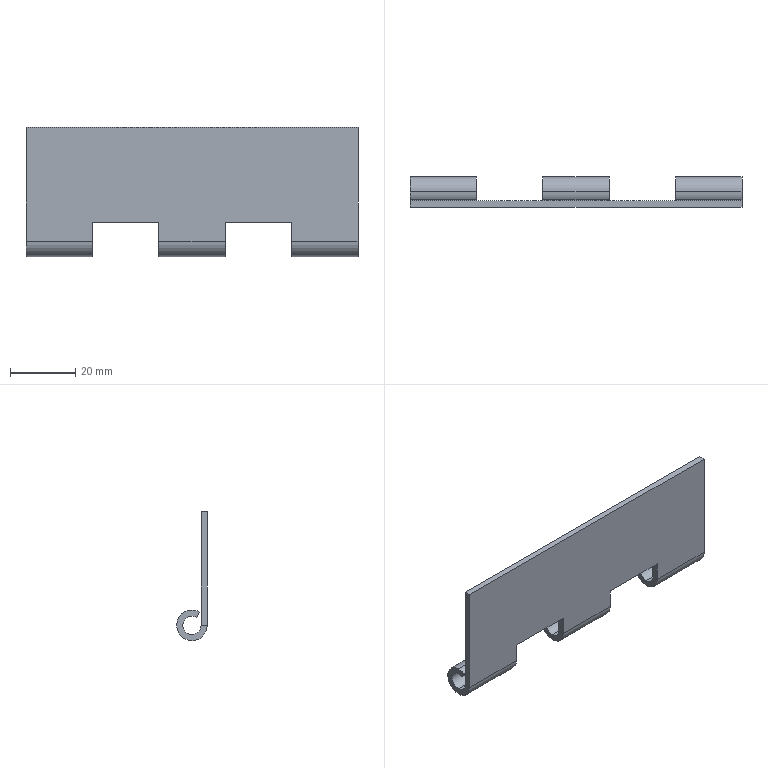Part | SolidWorks | features FlatPattern 1, ICE 1, SMBaseFlange 1, SheetMetal 1 | 1 solid | 36 faces | box 102 x 9.4 x 39.7 mm | volume 8617 mm3 | cylinder 18 | plane 18 | commonest cylinder face diameters 5.6 x9 9.4 x9
STEP:
#1=CARTESIAN_POINT('',(51.,1.9,-35.));
#2=VERTEX_POINT('',#1);
#3=CARTESIAN_POINT('',(51.,4.7,-37.8));
#4=VERTEX_POINT('',#3);
#5=CARTESIAN_POINT('',(51.,4.7,-35.));
#6=DIRECTION('',(1.,0.,0.));
#7=DIRECTION('',(0.,0.,-1.));
#8=AXIS2_PLACEMENT_3D('',#5,#6,#7);
#9=CIRCLE('',#8,2.8);
#10=EDGE_CURVE('',#2,#4,#9,.T.);
#11=ORIENTED_EDGE('',*,*,#10,.T.);
#12=CARTESIAN_POINT('',(30.6,4.7,-37.8));
#13=VERTEX_POINT('',#12);
#14=CARTESIAN_POINT('',(51.,4.7,-37.8));
#15=DIRECTION('',(-1.,0.,0.));
#16=VECTOR('',#15,1000.);
#17=LINE('',#14,#16);
#18=EDGE_CURVE('',#4,#13,#17,.T.);
#19=ORIENTED_EDGE('',*,*,#18,.T.);
#20=CARTESIAN_POINT('',(30.6,1.9,-35.));
#21=VERTEX_POINT('',#20);
#22=CARTESIAN_POINT('',(30.6,4.7,-35.));
#23=DIRECTION('',(1.,0.,0.));
#24=DIRECTION('',(0.,0.,-1.));
#25=AXIS2_PLACEMENT_3D('',#22,#23,#24);
#26=CIRCLE('',#25,2.8);
#27=EDGE_CURVE('',#21,#13,#26,.T.);
#28=ORIENTED_EDGE('',*,*,#27,.F.);
#29=CARTESIAN_POINT('',(51.,1.9,-35.));
#30=DIRECTION('',(-1.,0.,0.));
#31=VECTOR('',#30,1000.);
#32=LINE('',#29,#31);
#33=EDGE_CURVE('',#2,#21,#32,.T.);
#34=ORIENTED_EDGE('',*,*,#33,.F.);
#35=EDGE_LOOP('',(#11,#19,#28,#34));
#36=FACE_OUTER_BOUND('',#35,.T.);
#37=CARTESIAN_POINT('',(51.,4.7,-35.));
#38=DIRECTION('',(-1.,0.,0.));
#39=DIRECTION('',(0.,0.,1.));
#40=AXIS2_PLACEMENT_3D('',#37,#38,#39);
#41=CYLINDRICAL_SURFACE('',#40,2.8);
#42=ADVANCED_FACE('',(#36),#41,.F.);
#43=ORIENTED_EDGE('',*,*,#18,.F.);
#44=CARTESIAN_POINT('',(51.,4.7,-32.2));
#45=VERTEX_POINT('',#44);
#46=CARTESIAN_POINT('',(51.,4.7,-35.));
#47=DIRECTION('',(1.,0.,0.));
#48=DIRECTION('',(0.,0.,-1.));
#49=AXIS2_PLACEMENT_3D('',#46,#47,#48);
#50=CIRCLE('',#49,2.8);
#51=EDGE_CURVE('',#4,#45,#50,.T.);
#52=ORIENTED_EDGE('',*,*,#51,.T.);
#53=CARTESIAN_POINT('',(30.6,4.7,-32.2));
#54=VERTEX_POINT('',#53);
#55=CARTESIAN_POINT('',(51.,4.7,-32.2));
#56=DIRECTION('',(-1.,0.,0.));
#57=VECTOR('',#56,1000.);
#58=LINE('',#55,#57);
#59=EDGE_CURVE('',#45,#54,#58,.T.);
#60=ORIENTED_EDGE('',*,*,#59,.T.);
#61=CARTESIAN_POINT('',(30.6,4.7,-35.));
#62=DIRECTION('',(1.,0.,0.));
#63=DIRECTION('',(0.,0.,-1.));
#64=AXIS2_PLACEMENT_3D('',#61,#62,#63);
#65=CIRCLE('',#64,2.8);
#66=EDGE_CURVE('',#13,#54,#65,.T.);
#67=ORIENTED_EDGE('',*,*,#66,.F.);
#68=EDGE_LOOP('',(#43,#52,#60,#67));
#69=FACE_OUTER_BOUND('',#68,.T.);
#70=CARTESIAN_POINT('',(51.,4.7,-35.));
#71=DIRECTION('',(-1.,0.,0.));
#72=DIRECTION('',(0.,0.,1.));
#73=AXIS2_PLACEMENT_3D('',#70,#71,#72);
#74=CYLINDRICAL_SURFACE('',#73,2.8);
#75=ADVANCED_FACE('',(#69),#74,.F.);
#76=CARTESIAN_POINT('',(51.,4.7,-39.7));
#77=VERTEX_POINT('',#76);
#78=CARTESIAN_POINT('',(51.,4.7,-30.3));
#79=VERTEX_POINT('',#78);
#80=CARTESIAN_POINT('',(51.,4.7,-35.));
#81=DIRECTION('',(1.,0.,0.));
#82=DIRECTION('',(0.,0.,-1.));
#83=AXIS2_PLACEMENT_3D('',#80,#81,#82);
#84=CIRCLE('',#83,4.7);
#85=EDGE_CURVE('',#77,#79,#84,.T.);
#86=ORIENTED_EDGE('',*,*,#85,.F.);
#87=CARTESIAN_POINT('',(30.6,4.7,-39.7));
#88=VERTEX_POINT('',#87);
#89=CARTESIAN_POINT('',(51.,4.7,-39.7));
#90=DIRECTION('',(-1.,0.,0.));
#91=VECTOR('',#90,1000.);
#92=LINE('',#89,#91);
#93=EDGE_CURVE('',#77,#88,#92,.T.);
#94=ORIENTED_EDGE('',*,*,#93,.T.);
#95=CARTESIAN_POINT('',(30.6,4.7,-30.3));
#96=VERTEX_POINT('',#95);
#97=CARTESIAN_POINT('',(30.6,4.7,-35.));
#98=DIRECTION('',(1.,0.,0.));
#99=DIRECTION('',(0.,0.,-1.));
#100=AXIS2_PLACEMENT_3D('',#97,#98,#99);
#101=CIRCLE('',#100,4.7);
#102=EDGE_CURVE('',#88,#96,#101,.T.);
#103=ORIENTED_EDGE('',*,*,#102,.T.);
#104=CARTESIAN_POINT('',(51.,4.7,-30.3));
#105=DIRECTION('',(-1.,0.,0.));
#106=VECTOR('',#105,1000.);
#107=LINE('',#104,#106);
#108=EDGE_CURVE('',#79,#96,#107,.T.);
#109=ORIENTED_EDGE('',*,*,#108,.F.);
#110=EDGE_LOOP('',(#86,#94,#103,#109));
#111=FACE_OUTER_BOUND('',#110,.T.);
#112=CARTESIAN_POINT('',(51.,4.7,-35.));
#113=DIRECTION('',(-1.,0.,0.));
#114=DIRECTION('',(0.,0.,1.));
#115=AXIS2_PLACEMENT_3D('',#112,#113,#114);
#116=CYLINDRICAL_SURFACE('',#115,4.7);
#117=ADVANCED_FACE('',(#111),#116,.T.);
#118=CARTESIAN_POINT('',(51.,2.35,-30.93));
#119=VERTEX_POINT('',#118);
#120=CARTESIAN_POINT('',(51.,4.7,-35.));
#121=DIRECTION('',(1.,0.,0.));
#122=DIRECTION('',(0.,0.,-1.));
#123=AXIS2_PLACEMENT_3D('',#120,#121,#122);
#124=CIRCLE('',#123,4.7);
#125=EDGE_CURVE('',#79,#119,#124,.T.);
#126=ORIENTED_EDGE('',*,*,#125,.F.);
#127=ORIENTED_EDGE('',*,*,#108,.T.);
#128=CARTESIAN_POINT('',(30.6,2.35,-30.93));
#129=VERTEX_POINT('',#128);
#130=CARTESIAN_POINT('',(30.6,4.7,-35.));
#131=DIRECTION('',(1.,0.,0.));
#132=DIRECTION('',(0.,0.,-1.));
#133=AXIS2_PLACEMENT_3D('',#130,#131,#132);
#134=CIRCLE('',#133,4.7);
#135=EDGE_CURVE('',#96,#129,#134,.T.);
#136=ORIENTED_EDGE('',*,*,#135,.T.);
#137=CARTESIAN_POINT('',(51.,2.35,-30.93));
#138=DIRECTION('',(-1.,0.,0.));
#139=VECTOR('',#138,1000.);
#140=LINE('',#137,#139);
#141=EDGE_CURVE('',#119,#129,#140,.T.);
#142=ORIENTED_EDGE('',*,*,#141,.F.);
#143=EDGE_LOOP('',(#126,#127,#136,#142));
#144=FACE_OUTER_BOUND('',#143,.T.);
#145=CARTESIAN_POINT('',(51.,4.7,-35.));
#146=DIRECTION('',(-1.,0.,0.));
#147=DIRECTION('',(0.,0.,1.));
#148=AXIS2_PLACEMENT_3D('',#145,#146,#147);
#149=CYLINDRICAL_SURFACE('',#148,4.7);
#150=ADVANCED_FACE('',(#144),#149,.T.);
#151=CARTESIAN_POINT('',(10.2,4.7,-37.8));
#152=VERTEX_POINT('',#151);
#153=CARTESIAN_POINT('',(10.2,1.9,-35.));
#154=VERTEX_POINT('',#153);
#155=CARTESIAN_POINT('',(10.2,4.7,-35.));
#156=DIRECTION('',(-1.,0.,0.));
#157=DIRECTION('',(0.,0.,1.));
#158=AXIS2_PLACEMENT_3D('',#155,#156,#157);
#159=CIRCLE('',#158,2.8);
#160=EDGE_CURVE('',#152,#154,#159,.T.);
#161=ORIENTED_EDGE('',*,*,#160,.F.);
#162=CARTESIAN_POINT('',(-10.2,4.7,-37.8));
#163=VERTEX_POINT('',#162);
#164=CARTESIAN_POINT('',(51.,4.7,-37.8));
#165=DIRECTION('',(-1.,0.,0.));
#166=VECTOR('',#165,1000.);
#167=LINE('',#164,#166);
#168=EDGE_CURVE('',#152,#163,#167,.T.);
#169=ORIENTED_EDGE('',*,*,#168,.T.);
#170=CARTESIAN_POINT('',(-10.2,1.9,-35.));
#171=VERTEX_POINT('',#170);
#172=CARTESIAN_POINT('',(-10.2,4.7,-35.));
#173=DIRECTION('',(1.,0.,0.));
#174=DIRECTION('',(0.,0.,-1.));
#175=AXIS2_PLACEMENT_3D('',#172,#173,#174);
#176=CIRCLE('',#175,2.8);
#177=EDGE_CURVE('',#171,#163,#176,.T.);
#178=ORIENTED_EDGE('',*,*,#177,.F.);
#179=CARTESIAN_POINT('',(51.,1.9,-35.));
#180=DIRECTION('',(-1.,0.,0.));
#181=VECTOR('',#180,1000.);
#182=LINE('',#179,#181);
#183=EDGE_CURVE('',#154,#171,#182,.T.);
#184=ORIENTED_EDGE('',*,*,#183,.F.);
#185=EDGE_LOOP('',(#161,#169,#178,#184));
#186=FACE_OUTER_BOUND('',#185,.T.);
#187=CARTESIAN_POINT('',(51.,4.7,-35.));
#188=DIRECTION('',(-1.,0.,0.));
#189=DIRECTION('',(0.,0.,1.));
#190=AXIS2_PLACEMENT_3D('',#187,#188,#189);
#191=CYLINDRICAL_SURFACE('',#190,2.8);
#192=ADVANCED_FACE('',(#186),#191,.F.);
#193=ORIENTED_EDGE('',*,*,#168,.F.);
#194=CARTESIAN_POINT('',(10.2,4.7,-32.2));
#195=VERTEX_POINT('',#194);
#196=CARTESIAN_POINT('',(10.2,4.7,-35.));
#197=DIRECTION('',(-1.,0.,0.));
#198=DIRECTION('',(0.,0.,1.));
#199=AXIS2_PLACEMENT_3D('',#196,#197,#198);
#200=CIRCLE('',#199,2.8);
#201=EDGE_CURVE('',#195,#152,#200,.T.);
#202=ORIENTED_EDGE('',*,*,#201,.F.);
#203=CARTESIAN_POINT('',(-10.2,4.7,-32.2));
#204=VERTEX_POINT('',#203);
#205=CARTESIAN_POINT('',(51.,4.7,-32.2));
#206=DIRECTION('',(-1.,0.,0.));
#207=VECTOR('',#206,1000.);
#208=LINE('',#205,#207);
#209=EDGE_CURVE('',#195,#204,#208,.T.);
#210=ORIENTED_EDGE('',*,*,#209,.T.);
#211=CARTESIAN_POINT('',(-10.2,4.7,-35.));
#212=DIRECTION('',(1.,0.,0.));
#213=DIRECTION('',(0.,0.,-1.));
#214=AXIS2_PLACEMENT_3D('',#211,#212,#213);
#215=CIRCLE('',#214,2.8);
#216=EDGE_CURVE('',#163,#204,#215,.T.);
#217=ORIENTED_EDGE('',*,*,#216,.F.);
#218=EDGE_LOOP('',(#193,#202,#210,#217));
#219=FACE_OUTER_BOUND('',#218,.T.);
#220=CARTESIAN_POINT('',(51.,4.7,-35.));
#221=DIRECTION('',(-1.,0.,0.));
#222=DIRECTION('',(0.,0.,1.));
#223=AXIS2_PLACEMENT_3D('',#220,#221,#222);
#224=CYLINDRICAL_SURFACE('',#223,2.8);
#225=ADVANCED_FACE('',(#219),#224,.F.);
#226=CARTESIAN_POINT('',(-30.6,4.7,-37.8));
#227=VERTEX_POINT('',#226);
#228=CARTESIAN_POINT('',(-30.6,1.9,-35.));
#229=VERTEX_POINT('',#228);
#230=CARTESIAN_POINT('',(-30.6,4.7,-35.));
#231=DIRECTION('',(-1.,0.,0.));
#232=DIRECTION('',(0.,0.,1.));
#233=AXIS2_PLACEMENT_3D('',#230,#231,#232);
#234=CIRCLE('',#233,2.8);
#235=EDGE_CURVE('',#227,#229,#234,.T.);
#236=ORIENTED_EDGE('',*,*,#235,.F.);
#237=CARTESIAN_POINT('',(-51.,4.7,-37.8));
#238=VERTEX_POINT('',#237);
#239=CARTESIAN_POINT('',(51.,4.7,-37.8));
#240=DIRECTION('',(-1.,0.,0.));
#241=VECTOR('',#240,1000.);
#242=LINE('',#239,#241);
#243=EDGE_CURVE('',#227,#238,#242,.T.);
#244=ORIENTED_EDGE('',*,*,#243,.T.);
#245=CARTESIAN_POINT('',(-51.,1.9,-35.));
#246=VERTEX_POINT('',#245);
#247=CARTESIAN_POINT('',(-51.,4.7,-35.));
#248=DIRECTION('',(1.,0.,0.));
#249=DIRECTION('',(0.,0.,-1.));
#250=AXIS2_PLACEMENT_3D('',#247,#248,#249);
#251=CIRCLE('',#250,2.8);
#252=EDGE_CURVE('',#246,#238,#251,.T.);
#253=ORIENTED_EDGE('',*,*,#252,.F.);
#254=CARTESIAN_POINT('',(51.,1.9,-35.));
#255=DIRECTION('',(-1.,0.,0.));
#256=VECTOR('',#255,1000.);
#257=LINE('',#254,#256);
#258=EDGE_CURVE('',#229,#246,#257,.T.);
#259=ORIENTED_EDGE('',*,*,#258,.F.);
#260=EDGE_LOOP('',(#236,#244,#253,#259));
#261=FACE_OUTER_BOUND('',#260,.T.);
#262=CARTESIAN_POINT('',(51.,4.7,-35.));
#263=DIRECTION('',(-1.,0.,0.));
#264=DIRECTION('',(0.,0.,1.));
#265=AXIS2_PLACEMENT_3D('',#262,#263,#264);
#266=CYLINDRICAL_SURFACE('',#265,2.8);
#267=ADVANCED_FACE('',(#261),#266,.F.);
#268=ORIENTED_EDGE('',*,*,#243,.F.);
#269=CARTESIAN_POINT('',(-30.6,4.7,-32.2));
#270=VERTEX_POINT('',#269);
#271=CARTESIAN_POINT('',(-30.6,4.7,-35.));
#272=DIRECTION('',(-1.,0.,0.));
#273=DIRECTION('',(0.,0.,1.));
#274=AXIS2_PLACEMENT_3D('',#271,#272,#273);
#275=CIRCLE('',#274,2.8);
#276=EDGE_CURVE('',#270,#227,#275,.T.);
#277=ORIENTED_EDGE('',*,*,#276,.F.);
#278=CARTESIAN_POINT('',(-51.,4.7,-32.2));
#279=VERTEX_POINT('',#278);
#280=CARTESIAN_POINT('',(51.,4.7,-32.2));
#281=DIRECTION('',(-1.,0.,0.));
#282=VECTOR('',#281,1000.);
#283=LINE('',#280,#282);
#284=EDGE_CURVE('',#270,#279,#283,.T.);
#285=ORIENTED_EDGE('',*,*,#284,.T.);
#286=CARTESIAN_POINT('',(-51.,4.7,-35.));
#287=DIRECTION('',(1.,0.,0.));
#288=DIRECTION('',(0.,0.,-1.));
#289=AXIS2_PLACEMENT_3D('',#286,#287,#288);
#290=CIRCLE('',#289,2.8);
#291=EDGE_CURVE('',#238,#279,#290,.T.);
#292=ORIENTED_EDGE('',*,*,#291,.F.);
#293=EDGE_LOOP('',(#268,#277,#285,#292));
#294=FACE_OUTER_BOUND('',#293,.T.);
#295=CARTESIAN_POINT('',(51.,4.7,-35.));
#296=DIRECTION('',(-1.,0.,0.));
#297=DIRECTION('',(0.,0.,1.));
#298=AXIS2_PLACEMENT_3D('',#295,#296,#297);
#299=CYLINDRICAL_SURFACE('',#298,2.8);
#300=ADVANCED_FACE('',(#294),#299,.F.);
#301=CARTESIAN_POINT('',(10.2,4.7,-30.3));
#302=VERTEX_POINT('',#301);
#303=CARTESIAN_POINT('',(10.2,4.7,-39.7));
#304=VERTEX_POINT('',#303);
#305=CARTESIAN_POINT('',(10.2,4.7,-35.));
#306=DIRECTION('',(-1.,0.,0.));
#307=DIRECTION('',(0.,0.,1.));
#308=AXIS2_PLACEMENT_3D('',#305,#306,#307);
#309=CIRCLE('',#308,4.7);
#310=EDGE_CURVE('',#302,#304,#309,.T.);
#311=ORIENTED_EDGE('',*,*,#310,.T.);
#312=CARTESIAN_POINT('',(-10.2,4.7,-39.7));
#313=VERTEX_POINT('',#312);
#314=CARTESIAN_POINT('',(51.,4.7,-39.7));
#315=DIRECTION('',(-1.,0.,0.));
#316=VECTOR('',#315,1000.);
#317=LINE('',#314,#316);
#318=EDGE_CURVE('',#304,#313,#317,.T.);
#319=ORIENTED_EDGE('',*,*,#318,.T.);
#320=CARTESIAN_POINT('',(-10.2,4.7,-30.3));
#321=VERTEX_POINT('',#320);
#322=CARTESIAN_POINT('',(-10.2,4.7,-35.));
#323=DIRECTION('',(1.,0.,0.));
#324=DIRECTION('',(0.,0.,-1.));
#325=AXIS2_PLACEMENT_3D('',#322,#323,#324);
#326=CIRCLE('',#325,4.7);
#327=EDGE_CURVE('',#313,#321,#326,.T.);
#328=ORIENTED_EDGE('',*,*,#327,.T.);
#329=CARTESIAN_POINT('',(51.,4.7,-30.3));
#330=DIRECTION('',(-1.,0.,0.));
#331=VECTOR('',#330,1000.);
#332=LINE('',#329,#331);
#333=EDGE_CURVE('',#302,#321,#332,.T.);
#334=ORIENTED_EDGE('',*,*,#333,.F.);
#335=EDGE_LOOP('',(#311,#319,#328,#334));
#336=FACE_OUTER_BOUND('',#335,.T.);
#337=CARTESIAN_POINT('',(51.,4.7,-35.));
#338=DIRECTION('',(-1.,0.,0.));
#339=DIRECTION('',(0.,0.,1.));
#340=AXIS2_PLACEMENT_3D('',#337,#338,#339);
#341=CYLINDRICAL_SURFACE('',#340,4.7);
#342=ADVANCED_FACE('',(#336),#341,.T.);
#343=CARTESIAN_POINT('',(10.2,2.35,-30.93));
#344=VERTEX_POINT('',#343);
#345=CARTESIAN_POINT('',(10.2,4.7,-35.));
#346=DIRECTION('',(-1.,0.,0.));
#347=DIRECTION('',(0.,0.,1.));
#348=AXIS2_PLACEMENT_3D('',#345,#346,#347);
#349=CIRCLE('',#348,4.7);
#350=EDGE_CURVE('',#344,#302,#349,.T.);
#351=ORIENTED_EDGE('',*,*,#350,.T.);
#352=ORIENTED_EDGE('',*,*,#333,.T.);
#353=CARTESIAN_POINT('',(-10.2,2.35,-30.93));
#354=VERTEX_POINT('',#353);
#355=CARTESIAN_POINT('',(-10.2,4.7,-35.));
#356=DIRECTION('',(1.,0.,0.));
#357=DIRECTION('',(0.,0.,-1.));
#358=AXIS2_PLACEMENT_3D('',#355,#356,#357);
#359=CIRCLE('',#358,4.7);
#360=EDGE_CURVE('',#321,#354,#359,.T.);
#361=ORIENTED_EDGE('',*,*,#360,.T.);
#362=CARTESIAN_POINT('',(51.,2.35,-30.93));
#363=DIRECTION('',(-1.,0.,0.));
#364=VECTOR('',#363,1000.);
#365=LINE('',#362,#364);
#366=EDGE_CURVE('',#344,#354,#365,.T.);
#367=ORIENTED_EDGE('',*,*,#366,.F.);
#368=EDGE_LOOP('',(#351,#352,#361,#367));
#369=FACE_OUTER_BOUND('',#368,.T.);
#370=CARTESIAN_POINT('',(51.,4.7,-35.));
#371=DIRECTION('',(-1.,0.,0.));
#372=DIRECTION('',(0.,0.,1.));
#373=AXIS2_PLACEMENT_3D('',#370,#371,#372);
#374=CYLINDRICAL_SURFACE('',#373,4.7);
#375=ADVANCED_FACE('',(#369),#374,.T.);
#376=CARTESIAN_POINT('',(-30.6,4.7,-30.3));
#377=VERTEX_POINT('',#376);
#378=CARTESIAN_POINT('',(-30.6,4.7,-39.7));
#379=VERTEX_POINT('',#378);
#380=CARTESIAN_POINT('',(-30.6,4.7,-35.));
#381=DIRECTION('',(-1.,0.,0.));
#382=DIRECTION('',(0.,0.,1.));
#383=AXIS2_PLACEMENT_3D('',#380,#381,#382);
#384=CIRCLE('',#383,4.7);
#385=EDGE_CURVE('',#377,#379,#384,.T.);
#386=ORIENTED_EDGE('',*,*,#385,.T.);
#387=CARTESIAN_POINT('',(-51.,4.7,-39.7));
#388=VERTEX_POINT('',#387);
#389=CARTESIAN_POINT('',(51.,4.7,-39.7));
#390=DIRECTION('',(-1.,0.,0.));
#391=VECTOR('',#390,1000.);
#392=LINE('',#389,#391);
#393=EDGE_CURVE('',#379,#388,#392,.T.);
#394=ORIENTED_EDGE('',*,*,#393,.T.);
#395=CARTESIAN_POINT('',(-51.,4.7,-30.3));
#396=VERTEX_POINT('',#395);
#397=CARTESIAN_POINT('',(-51.,4.7,-35.));
#398=DIRECTION('',(1.,0.,0.));
#399=DIRECTION('',(0.,0.,-1.));
#400=AXIS2_PLACEMENT_3D('',#397,#398,#399);
#401=CIRCLE('',#400,4.7);
#402=EDGE_CURVE('',#388,#396,#401,.T.);
#403=ORIENTED_EDGE('',*,*,#402,.T.);
#404=CARTESIAN_POINT('',(51.,4.7,-30.3));
#405=DIRECTION('',(-1.,0.,0.));
#406=VECTOR('',#405,1000.);
#407=LINE('',#404,#406);
#408=EDGE_CURVE('',#377,#396,#407,.T.);
#409=ORIENTED_EDGE('',*,*,#408,.F.);
#410=EDGE_LOOP('',(#386,#394,#403,#409));
#411=FACE_OUTER_BOUND('',#410,.T.);
#412=CARTESIAN_POINT('',(51.,4.7,-35.));
#413=DIRECTION('',(-1.,0.,0.));
#414=DIRECTION('',(0.,0.,1.));
#415=AXIS2_PLACEMENT_3D('',#412,#413,#414);
#416=CYLINDRICAL_SURFACE('',#415,4.7);
#417=ADVANCED_FACE('',(#411),#416,.T.);
#418=CARTESIAN_POINT('',(-30.6,2.35,-30.93));
#419=VERTEX_POINT('',#418);
#420=CARTESIAN_POINT('',(-30.6,4.7,-35.));
#421=DIRECTION('',(-1.,0.,0.));
#422=DIRECTION('',(0.,0.,1.));
#423=AXIS2_PLACEMENT_3D('',#420,#421,#422);
#424=CIRCLE('',#423,4.7);
#425=EDGE_CURVE('',#419,#377,#424,.T.);
#426=ORIENTED_EDGE('',*,*,#425,.T.);
#427=ORIENTED_EDGE('',*,*,#408,.T.);
#428=CARTESIAN_POINT('',(-51.,2.35,-30.93));
#429=VERTEX_POINT('',#428);
#430=CARTESIAN_POINT('',(-51.,4.7,-35.));
#431=DIRECTION('',(1.,0.,0.));
#432=DIRECTION('',(0.,0.,-1.));
#433=AXIS2_PLACEMENT_3D('',#430,#431,#432);
#434=CIRCLE('',#433,4.7);
#435=EDGE_CURVE('',#396,#429,#434,.T.);
#436=ORIENTED_EDGE('',*,*,#435,.T.);
#437=CARTESIAN_POINT('',(51.,2.35,-30.93));
#438=DIRECTION('',(-1.,0.,0.));
#439=VECTOR('',#438,1000.);
#440=LINE('',#437,#439);
#441=EDGE_CURVE('',#419,#429,#440,.T.);
#442=ORIENTED_EDGE('',*,*,#441,.F.);
#443=EDGE_LOOP('',(#426,#427,#436,#442));
#444=FACE_OUTER_BOUND('',#443,.T.);
#445=CARTESIAN_POINT('',(51.,4.7,-35.));
#446=DIRECTION('',(-1.,0.,0.));
#447=DIRECTION('',(0.,0.,1.));
#448=AXIS2_PLACEMENT_3D('',#445,#446,#447);
#449=CYLINDRICAL_SURFACE('',#448,4.7);
#450=ADVANCED_FACE('',(#444),#449,.T.);
#451=CARTESIAN_POINT('',(-10.2,1.9,-29.2));
#452=VERTEX_POINT('',#451);
#453=CARTESIAN_POINT('',(-10.2,1.9,0.));
#454=DIRECTION('',(0.,0.,-1.));
#455=VECTOR('',#454,1000.);
#456=LINE('',#453,#455);
#457=EDGE_CURVE('',#452,#171,#456,.T.);
#458=ORIENTED_EDGE('',*,*,#457,.T.);
#459=CARTESIAN_POINT('',(-10.2,0.,-35.));
#460=VERTEX_POINT('',#459);
#461=CARTESIAN_POINT('',(-10.2,1.9,-35.));
#462=DIRECTION('',(0.,-1.,0.));
#463=VECTOR('',#462,1000.);
#464=LINE('',#461,#463);
#465=EDGE_CURVE('',#171,#460,#464,.T.);
#466=ORIENTED_EDGE('',*,*,#465,.T.);
#467=CARTESIAN_POINT('',(-10.2,0.,-29.2));
#468=VERTEX_POINT('',#467);
#469=CARTESIAN_POINT('',(-10.2,0.,0.));
#470=DIRECTION('',(0.,0.,-1.));
#471=VECTOR('',#470,1000.);
#472=LINE('',#469,#471);
#473=EDGE_CURVE('',#468,#460,#472,.T.);
#474=ORIENTED_EDGE('',*,*,#473,.F.);
#475=CARTESIAN_POINT('',(-10.2,9.4,-29.2));
#476=DIRECTION('',(0.,-1.,0.));
#477=VECTOR('',#476,1000.);
#478=LINE('',#475,#477);
#479=EDGE_CURVE('',#452,#468,#478,.T.);
#480=ORIENTED_EDGE('',*,*,#479,.F.);
#481=EDGE_LOOP('',(#458,#466,#474,#480));
#482=FACE_OUTER_BOUND('',#481,.T.);
#483=CARTESIAN_POINT('',(-10.2,9.4,-39.7));
#484=DIRECTION('',(1.,0.,0.));
#485=DIRECTION('',(0.,0.,-1.));
#486=AXIS2_PLACEMENT_3D('',#483,#484,#485);
#487=PLANE('',#486);
#488=ADVANCED_FACE('',(#482),#487,.F.);
#489=CARTESIAN_POINT('',(30.6,1.9,-29.2));
#490=VERTEX_POINT('',#489);
#491=CARTESIAN_POINT('',(30.6,1.9,0.));
#492=DIRECTION('',(0.,0.,-1.));
#493=VECTOR('',#492,1000.);
#494=LINE('',#491,#493);
#495=EDGE_CURVE('',#490,#21,#494,.T.);
#496=ORIENTED_EDGE('',*,*,#495,.T.);
#497=CARTESIAN_POINT('',(30.6,0.,-35.));
#498=VERTEX_POINT('',#497);
#499=CARTESIAN_POINT('',(30.6,1.9,-35.));
#500=DIRECTION('',(0.,-1.,0.));
#501=VECTOR('',#500,1000.);
#502=LINE('',#499,#501);
#503=EDGE_CURVE('',#21,#498,#502,.T.);
#504=ORIENTED_EDGE('',*,*,#503,.T.);
#505=CARTESIAN_POINT('',(30.6,0.,-29.2));
#506=VERTEX_POINT('',#505);
#507=CARTESIAN_POINT('',(30.6,0.,0.));
#508=DIRECTION('',(0.,0.,-1.));
#509=VECTOR('',#508,1000.);
#510=LINE('',#507,#509);
#511=EDGE_CURVE('',#506,#498,#510,.T.);
#512=ORIENTED_EDGE('',*,*,#511,.F.);
#513=CARTESIAN_POINT('',(30.6,9.4,-29.2));
#514=DIRECTION('',(0.,-1.,0.));
#515=VECTOR('',#514,1000.);
#516=LINE('',#513,#515);
#517=EDGE_CURVE('',#490,#506,#516,.T.);
#518=ORIENTED_EDGE('',*,*,#517,.F.);
#519=EDGE_LOOP('',(#496,#504,#512,#518));
#520=FACE_OUTER_BOUND('',#519,.T.);
#521=CARTESIAN_POINT('',(30.6,9.4,-39.7));
#522=DIRECTION('',(1.,0.,0.));
#523=DIRECTION('',(0.,0.,-1.));
#524=AXIS2_PLACEMENT_3D('',#521,#522,#523);
#525=PLANE('',#524);
#526=ADVANCED_FACE('',(#520),#525,.F.);
#527=ORIENTED_EDGE('',*,*,#393,.F.);
#528=CARTESIAN_POINT('',(-30.6,0.,-35.));
#529=VERTEX_POINT('',#528);
#530=CARTESIAN_POINT('',(-30.6,4.7,-35.));
#531=DIRECTION('',(-1.,0.,0.));
#532=DIRECTION('',(0.,0.,1.));
#533=AXIS2_PLACEMENT_3D('',#530,#531,#532);
#534=CIRCLE('',#533,4.7);
#535=EDGE_CURVE('',#379,#529,#534,.T.);
#536=ORIENTED_EDGE('',*,*,#535,.T.);
#537=CARTESIAN_POINT('',(-51.,0.,-35.));
#538=VERTEX_POINT('',#537);
#539=CARTESIAN_POINT('',(51.,0.,-35.));
#540=DIRECTION('',(-1.,0.,0.));
#541=VECTOR('',#540,1000.);
#542=LINE('',#539,#541);
#543=EDGE_CURVE('',#529,#538,#542,.T.);
#544=ORIENTED_EDGE('',*,*,#543,.T.);
#545=CARTESIAN_POINT('',(-51.,4.7,-35.));
#546=DIRECTION('',(1.,0.,0.));
#547=DIRECTION('',(0.,0.,-1.));
#548=AXIS2_PLACEMENT_3D('',#545,#546,#547);
#549=CIRCLE('',#548,4.7);
#550=EDGE_CURVE('',#538,#388,#549,.T.);
#551=ORIENTED_EDGE('',*,*,#550,.T.);
#552=EDGE_LOOP('',(#527,#536,#544,#551));
#553=FACE_OUTER_BOUND('',#552,.T.);
#554=CARTESIAN_POINT('',(51.,4.7,-35.));
#555=DIRECTION('',(-1.,0.,0.));
#556=DIRECTION('',(0.,0.,1.));
#557=AXIS2_PLACEMENT_3D('',#554,#555,#556);
#558=CYLINDRICAL_SURFACE('',#557,4.7);
#559=ADVANCED_FACE('',(#553),#558,.T.);
#560=ORIENTED_EDGE('',*,*,#318,.F.);
#561=CARTESIAN_POINT('',(10.2,0.,-35.));
#562=VERTEX_POINT('',#561);
#563=CARTESIAN_POINT('',(10.2,4.7,-35.));
#564=DIRECTION('',(-1.,0.,0.));
#565=DIRECTION('',(0.,0.,1.));
#566=AXIS2_PLACEMENT_3D('',#563,#564,#565);
#567=CIRCLE('',#566,4.7);
#568=EDGE_CURVE('',#304,#562,#567,.T.);
#569=ORIENTED_EDGE('',*,*,#568,.T.);
#570=CARTESIAN_POINT('',(51.,0.,-35.));
#571=DIRECTION('',(-1.,0.,0.));
#572=VECTOR('',#571,1000.);
#573=LINE('',#570,#572);
#574=EDGE_CURVE('',#562,#460,#573,.T.);
#575=ORIENTED_EDGE('',*,*,#574,.T.);
#576=CARTESIAN_POINT('',(-10.2,4.7,-35.));
#577=DIRECTION('',(1.,0.,0.));
#578=DIRECTION('',(0.,0.,-1.));
#579=AXIS2_PLACEMENT_3D('',#576,#577,#578);
#580=CIRCLE('',#579,4.7);
#581=EDGE_CURVE('',#460,#313,#580,.T.);
#582=ORIENTED_EDGE('',*,*,#581,.T.);
#583=EDGE_LOOP('',(#560,#569,#575,#582));
#584=FACE_OUTER_BOUND('',#583,.T.);
#585=CARTESIAN_POINT('',(51.,4.7,-35.));
#586=DIRECTION('',(-1.,0.,0.));
#587=DIRECTION('',(0.,0.,1.));
#588=AXIS2_PLACEMENT_3D('',#585,#586,#587);
#589=CYLINDRICAL_SURFACE('',#588,4.7);
#590=ADVANCED_FACE('',(#584),#589,.T.);
#591=CARTESIAN_POINT('',(-30.6,3.3,-32.575));
#592=VERTEX_POINT('',#591);
#593=CARTESIAN_POINT('',(-30.6,3.3,-32.575));
#594=DIRECTION('',(0.,0.5,-0.866));
#595=VECTOR('',#594,1000.);
#596=LINE('',#593,#595);
#597=EDGE_CURVE('',#419,#592,#596,.T.);
#598=ORIENTED_EDGE('',*,*,#597,.F.);
#599=ORIENTED_EDGE('',*,*,#441,.T.);
#600=CARTESIAN_POINT('',(-51.,3.3,-32.575));
#601=VERTEX_POINT('',#600);
#602=CARTESIAN_POINT('',(-51.,3.3,-32.575));
#603=DIRECTION('',(0.,-0.5,0.866));
#604=VECTOR('',#603,1000.);
#605=LINE('',#602,#604);
#606=EDGE_CURVE('',#601,#429,#605,.T.);
#607=ORIENTED_EDGE('',*,*,#606,.F.);
#608=CARTESIAN_POINT('',(51.,3.3,-32.575));
#609=DIRECTION('',(-1.,0.,0.));
#610=VECTOR('',#609,1000.);
#611=LINE('',#608,#610);
#612=EDGE_CURVE('',#592,#601,#611,.T.);
#613=ORIENTED_EDGE('',*,*,#612,.F.);
#614=EDGE_LOOP('',(#598,#599,#607,#613));
#615=FACE_OUTER_BOUND('',#614,.T.);
#616=CARTESIAN_POINT('',(51.,3.3,-32.575));
#617=DIRECTION('',(0.,-0.866,-0.5));
#618=DIRECTION('',(0.,0.5,-0.866));
#619=AXIS2_PLACEMENT_3D('',#616,#617,#618);
#620=PLANE('',#619);
#621=ADVANCED_FACE('',(#615),#620,.T.);
#622=CARTESIAN_POINT('',(-10.2,3.3,-32.575));
#623=VERTEX_POINT('',#622);
#624=CARTESIAN_POINT('',(-10.2,3.3,-32.575));
#625=DIRECTION('',(0.,-0.5,0.866));
#626=VECTOR('',#625,1000.);
#627=LINE('',#624,#626);
#628=EDGE_CURVE('',#623,#354,#627,.T.);
#629=ORIENTED_EDGE('',*,*,#628,.F.);
#630=CARTESIAN_POINT('',(10.2,3.3,-32.575));
#631=VERTEX_POINT('',#630);
#632=CARTESIAN_POINT('',(51.,3.3,-32.575));
#633=DIRECTION('',(-1.,0.,0.));
#634=VECTOR('',#633,1000.);
#635=LINE('',#632,#634);
#636=EDGE_CURVE('',#631,#623,#635,.T.);
#637=ORIENTED_EDGE('',*,*,#636,.F.);
#638=CARTESIAN_POINT('',(10.2,3.3,-32.575));
#639=DIRECTION('',(0.,0.5,-0.866));
#640=VECTOR('',#639,1000.);
#641=LINE('',#638,#640);
#642=EDGE_CURVE('',#344,#631,#641,.T.);
#643=ORIENTED_EDGE('',*,*,#642,.F.);
#644=ORIENTED_EDGE('',*,*,#366,.T.);
#645=EDGE_LOOP('',(#629,#637,#643,#644));
#646=FACE_OUTER_BOUND('',#645,.T.);
#647=CARTESIAN_POINT('',(51.,3.3,-32.575));
#648=DIRECTION('',(0.,-0.866,-0.5));
#649=DIRECTION('',(0.,0.5,-0.866));
#650=AXIS2_PLACEMENT_3D('',#647,#648,#649);
#651=PLANE('',#650);
#652=ADVANCED_FACE('',(#646),#651,.T.);
#653=ORIENTED_EDGE('',*,*,#284,.F.);
#654=CARTESIAN_POINT('',(-30.6,4.7,-35.));
#655=DIRECTION('',(-1.,0.,0.));
#656=DIRECTION('',(0.,0.,1.));
#657=AXIS2_PLACEMENT_3D('',#654,#655,#656);
#658=CIRCLE('',#657,2.8);
#659=EDGE_CURVE('',#592,#270,#658,.T.);
#660=ORIENTED_EDGE('',*,*,#659,.F.);
#661=ORIENTED_EDGE('',*,*,#612,.T.);
#662=CARTESIAN_POINT('',(-51.,4.7,-35.));
#663=DIRECTION('',(1.,0.,0.));
#664=DIRECTION('',(0.,0.,-1.));
#665=AXIS2_PLACEMENT_3D('',#662,#663,#664);
#666=CIRCLE('',#665,2.8);
#667=EDGE_CURVE('',#279,#601,#666,.T.);
#668=ORIENTED_EDGE('',*,*,#667,.F.);
#669=EDGE_LOOP('',(#653,#660,#661,#668));
#670=FACE_OUTER_BOUND('',#669,.T.);
#671=CARTESIAN_POINT('',(51.,4.7,-35.));
#672=DIRECTION('',(-1.,0.,0.));
#673=DIRECTION('',(0.,0.,1.));
#674=AXIS2_PLACEMENT_3D('',#671,#672,#673);
#675=CYLINDRICAL_SURFACE('',#674,2.8);
#676=ADVANCED_FACE('',(#670),#675,.F.);
#677=ORIENTED_EDGE('',*,*,#209,.F.);
#678=CARTESIAN_POINT('',(10.2,4.7,-35.));
#679=DIRECTION('',(-1.,0.,0.));
#680=DIRECTION('',(0.,0.,1.));
#681=AXIS2_PLACEMENT_3D('',#678,#679,#680);
#682=CIRCLE('',#681,2.8);
#683=EDGE_CURVE('',#631,#195,#682,.T.);
#684=ORIENTED_EDGE('',*,*,#683,.F.);
#685=ORIENTED_EDGE('',*,*,#636,.T.);
#686=CARTESIAN_POINT('',(-10.2,4.7,-35.));
#687=DIRECTION('',(1.,0.,0.));
#688=DIRECTION('',(0.,0.,-1.));
#689=AXIS2_PLACEMENT_3D('',#686,#687,#688);
#690=CIRCLE('',#689,2.8);
#691=EDGE_CURVE('',#204,#623,#690,.T.);
#692=ORIENTED_EDGE('',*,*,#691,.F.);
#693=EDGE_LOOP('',(#677,#684,#685,#692));
#694=FACE_OUTER_BOUND('',#693,.T.);
#695=CARTESIAN_POINT('',(51.,4.7,-35.));
#696=DIRECTION('',(-1.,0.,0.));
#697=DIRECTION('',(0.,0.,1.));
#698=AXIS2_PLACEMENT_3D('',#695,#696,#697);
#699=CYLINDRICAL_SURFACE('',#698,2.8);
#700=ADVANCED_FACE('',(#694),#699,.F.);
#701=CARTESIAN_POINT('',(51.,0.,-35.));
#702=VERTEX_POINT('',#701);
#703=CARTESIAN_POINT('',(51.,0.,-35.));
#704=DIRECTION('',(0.,1.,0.));
#705=VECTOR('',#704,1000.);
#706=LINE('',#703,#705);
#707=EDGE_CURVE('',#702,#2,#706,.T.);
#708=ORIENTED_EDGE('',*,*,#707,.F.);
#709=CARTESIAN_POINT('',(51.,4.7,-35.));
#710=DIRECTION('',(1.,0.,0.));
#711=DIRECTION('',(0.,0.,-1.));
#712=AXIS2_PLACEMENT_3D('',#709,#710,#711);
#713=CIRCLE('',#712,4.7);
#714=EDGE_CURVE('',#702,#77,#713,.T.);
#715=ORIENTED_EDGE('',*,*,#714,.T.);
#716=ORIENTED_EDGE('',*,*,#85,.T.);
#717=ORIENTED_EDGE('',*,*,#125,.T.);
#718=CARTESIAN_POINT('',(51.,3.3,-32.575));
#719=VERTEX_POINT('',#718);
#720=CARTESIAN_POINT('',(51.,3.3,-32.575));
#721=DIRECTION('',(0.,-0.5,0.866));
#722=VECTOR('',#721,1000.);
#723=LINE('',#720,#722);
#724=EDGE_CURVE('',#719,#119,#723,.T.);
#725=ORIENTED_EDGE('',*,*,#724,.F.);
#726=CARTESIAN_POINT('',(51.,4.7,-35.));
#727=DIRECTION('',(1.,0.,0.));
#728=DIRECTION('',(0.,0.,-1.));
#729=AXIS2_PLACEMENT_3D('',#726,#727,#728);
#730=CIRCLE('',#729,2.8);
#731=EDGE_CURVE('',#45,#719,#730,.T.);
#732=ORIENTED_EDGE('',*,*,#731,.F.);
#733=ORIENTED_EDGE('',*,*,#51,.F.);
#734=ORIENTED_EDGE('',*,*,#10,.F.);
#735=EDGE_LOOP('',(#708,#715,#716,#717,#725,#732,#733,#734));
#736=FACE_OUTER_BOUND('',#735,.T.);
#737=CARTESIAN_POINT('',(51.,0.,-35.));
#738=DIRECTION('',(1.,0.,0.));
#739=DIRECTION('',(0.,0.,-1.));
#740=AXIS2_PLACEMENT_3D('',#737,#738,#739);
#741=PLANE('',#740);
#742=ADVANCED_FACE('',(#736),#741,.T.);
#743=CARTESIAN_POINT('',(-51.,1.9,-35.));
#744=DIRECTION('',(0.,-1.,0.));
#745=VECTOR('',#744,1000.);
#746=LINE('',#743,#745);
#747=EDGE_CURVE('',#246,#538,#746,.T.);
#748=ORIENTED_EDGE('',*,*,#747,.F.);
#749=ORIENTED_EDGE('',*,*,#252,.T.);
#750=ORIENTED_EDGE('',*,*,#291,.T.);
#751=ORIENTED_EDGE('',*,*,#667,.T.);
#752=ORIENTED_EDGE('',*,*,#606,.T.);
#753=ORIENTED_EDGE('',*,*,#435,.F.);
#754=ORIENTED_EDGE('',*,*,#402,.F.);
#755=ORIENTED_EDGE('',*,*,#550,.F.);
#756=EDGE_LOOP('',(#748,#749,#750,#751,#752,#753,#754,#755));
#757=FACE_OUTER_BOUND('',#756,.T.);
#758=CARTESIAN_POINT('',(-51.,1.9,-35.));
#759=DIRECTION('',(-1.,0.,0.));
#760=DIRECTION('',(0.,0.,1.));
#761=AXIS2_PLACEMENT_3D('',#758,#759,#760);
#762=PLANE('',#761);
#763=ADVANCED_FACE('',(#757),#762,.T.);
#764=ORIENTED_EDGE('',*,*,#93,.F.);
#765=ORIENTED_EDGE('',*,*,#714,.F.);
#766=CARTESIAN_POINT('',(51.,0.,-35.));
#767=DIRECTION('',(-1.,0.,0.));
#768=VECTOR('',#767,1000.);
#769=LINE('',#766,#768);
#770=EDGE_CURVE('',#702,#498,#769,.T.);
#771=ORIENTED_EDGE('',*,*,#770,.T.);
#772=CARTESIAN_POINT('',(30.6,4.7,-35.));
#773=DIRECTION('',(1.,0.,0.));
#774=DIRECTION('',(0.,0.,-1.));
#775=AXIS2_PLACEMENT_3D('',#772,#773,#774);
#776=CIRCLE('',#775,4.7);
#777=EDGE_CURVE('',#498,#88,#776,.T.);
#778=ORIENTED_EDGE('',*,*,#777,.T.);
#779=EDGE_LOOP('',(#764,#765,#771,#778));
#780=FACE_OUTER_BOUND('',#779,.T.);
#781=CARTESIAN_POINT('',(51.,4.7,-35.));
#782=DIRECTION('',(-1.,0.,0.));
#783=DIRECTION('',(0.,0.,1.));
#784=AXIS2_PLACEMENT_3D('',#781,#782,#783);
#785=CYLINDRICAL_SURFACE('',#784,4.7);
#786=ADVANCED_FACE('',(#780),#785,.T.);
#787=CARTESIAN_POINT('',(30.6,3.3,-32.575));
#788=VERTEX_POINT('',#787);
#789=CARTESIAN_POINT('',(30.6,3.3,-32.575));
#790=DIRECTION('',(0.,-0.5,0.866));
#791=VECTOR('',#790,1000.);
#792=LINE('',#789,#791);
#793=EDGE_CURVE('',#788,#129,#792,.T.);
#794=ORIENTED_EDGE('',*,*,#793,.F.);
#795=CARTESIAN_POINT('',(51.,3.3,-32.575));
#796=DIRECTION('',(-1.,0.,0.));
#797=VECTOR('',#796,1000.);
#798=LINE('',#795,#797);
#799=EDGE_CURVE('',#719,#788,#798,.T.);
#800=ORIENTED_EDGE('',*,*,#799,.F.);
#801=ORIENTED_EDGE('',*,*,#724,.T.);
#802=ORIENTED_EDGE('',*,*,#141,.T.);
#803=EDGE_LOOP('',(#794,#800,#801,#802));
#804=FACE_OUTER_BOUND('',#803,.T.);
#805=CARTESIAN_POINT('',(51.,3.3,-32.575));
#806=DIRECTION('',(0.,-0.866,-0.5));
#807=DIRECTION('',(0.,0.5,-0.866));
#808=AXIS2_PLACEMENT_3D('',#805,#806,#807);
#809=PLANE('',#808);
#810=ADVANCED_FACE('',(#804),#809,.T.);
#811=ORIENTED_EDGE('',*,*,#59,.F.);
#812=ORIENTED_EDGE('',*,*,#731,.T.);
#813=ORIENTED_EDGE('',*,*,#799,.T.);
#814=CARTESIAN_POINT('',(30.6,4.7,-35.));
#815=DIRECTION('',(1.,0.,0.));
#816=DIRECTION('',(0.,0.,-1.));
#817=AXIS2_PLACEMENT_3D('',#814,#815,#816);
#818=CIRCLE('',#817,2.8);
#819=EDGE_CURVE('',#54,#788,#818,.T.);
#820=ORIENTED_EDGE('',*,*,#819,.F.);
#821=EDGE_LOOP('',(#811,#812,#813,#820));
#822=FACE_OUTER_BOUND('',#821,.T.);
#823=CARTESIAN_POINT('',(51.,4.7,-35.));
#824=DIRECTION('',(-1.,0.,0.));
#825=DIRECTION('',(0.,0.,1.));
#826=AXIS2_PLACEMENT_3D('',#823,#824,#825);
#827=CYLINDRICAL_SURFACE('',#826,2.8);
#828=ADVANCED_FACE('',(#822),#827,.F.);
#829=CARTESIAN_POINT('',(-30.6,1.9,-29.2));
#830=VERTEX_POINT('',#829);
#831=CARTESIAN_POINT('',(-30.6,1.9,0.));
#832=DIRECTION('',(0.,0.,1.));
#833=VECTOR('',#832,1000.);
#834=LINE('',#831,#833);
#835=EDGE_CURVE('',#229,#830,#834,.T.);
#836=ORIENTED_EDGE('',*,*,#835,.F.);
#837=ORIENTED_EDGE('',*,*,#258,.T.);
#838=CARTESIAN_POINT('',(-51.,1.9,0.));
#839=VERTEX_POINT('',#838);
#840=CARTESIAN_POINT('',(-51.,1.9,0.));
#841=DIRECTION('',(0.,0.,-1.));
#842=VECTOR('',#841,1000.);
#843=LINE('',#840,#842);
#844=EDGE_CURVE('',#839,#246,#843,.T.);
#845=ORIENTED_EDGE('',*,*,#844,.F.);
#846=CARTESIAN_POINT('',(51.,1.9,0.));
#847=VERTEX_POINT('',#846);
#848=CARTESIAN_POINT('',(51.,1.9,0.));
#849=DIRECTION('',(-1.,0.,0.));
#850=VECTOR('',#849,1000.);
#851=LINE('',#848,#850);
#852=EDGE_CURVE('',#847,#839,#851,.T.);
#853=ORIENTED_EDGE('',*,*,#852,.F.);
#854=CARTESIAN_POINT('',(51.,1.9,0.));
#855=DIRECTION('',(0.,0.,-1.));
#856=VECTOR('',#855,1000.);
#857=LINE('',#854,#856);
#858=EDGE_CURVE('',#847,#2,#857,.T.);
#859=ORIENTED_EDGE('',*,*,#858,.T.);
#860=ORIENTED_EDGE('',*,*,#33,.T.);
#861=ORIENTED_EDGE('',*,*,#495,.F.);
#862=CARTESIAN_POINT('',(10.2,1.9,-29.2));
#863=VERTEX_POINT('',#862);
#864=CARTESIAN_POINT('',(51.,1.9,-29.2));
#865=DIRECTION('',(1.,0.,0.));
#866=VECTOR('',#865,1000.);
#867=LINE('',#864,#866);
#868=EDGE_CURVE('',#863,#490,#867,.T.);
#869=ORIENTED_EDGE('',*,*,#868,.F.);
#870=CARTESIAN_POINT('',(10.2,1.9,0.));
#871=DIRECTION('',(0.,0.,1.));
#872=VECTOR('',#871,1000.);
#873=LINE('',#870,#872);
#874=EDGE_CURVE('',#154,#863,#873,.T.);
#875=ORIENTED_EDGE('',*,*,#874,.F.);
#876=ORIENTED_EDGE('',*,*,#183,.T.);
#877=ORIENTED_EDGE('',*,*,#457,.F.);
#878=CARTESIAN_POINT('',(51.,1.9,-29.2));
#879=DIRECTION('',(1.,0.,0.));
#880=VECTOR('',#879,1000.);
#881=LINE('',#878,#880);
#882=EDGE_CURVE('',#830,#452,#881,.T.);
#883=ORIENTED_EDGE('',*,*,#882,.F.);
#884=EDGE_LOOP('',(#836,#837,#845,#853,#859,#860,#861,#869,#875,#876,#877,#883));
#885=FACE_OUTER_BOUND('',#884,.T.);
#886=CARTESIAN_POINT('',(51.,1.9,0.));
#887=DIRECTION('',(0.,1.,0.));
#888=DIRECTION('',(0.,0.,1.));
#889=AXIS2_PLACEMENT_3D('',#886,#887,#888);
#890=PLANE('',#889);
#891=ADVANCED_FACE('',(#885),#890,.T.);
#892=CARTESIAN_POINT('',(-51.,0.,0.));
#893=VERTEX_POINT('',#892);
#894=CARTESIAN_POINT('',(-51.,0.,0.));
#895=DIRECTION('',(0.,1.,0.));
#896=VECTOR('',#895,1000.);
#897=LINE('',#894,#896);
#898=EDGE_CURVE('',#893,#839,#897,.T.);
#899=ORIENTED_EDGE('',*,*,#898,.F.);
#900=CARTESIAN_POINT('',(51.,0.,0.));
#901=VERTEX_POINT('',#900);
#902=CARTESIAN_POINT('',(51.,0.,0.));
#903=DIRECTION('',(-1.,0.,0.));
#904=VECTOR('',#903,1000.);
#905=LINE('',#902,#904);
#906=EDGE_CURVE('',#901,#893,#905,.T.);
#907=ORIENTED_EDGE('',*,*,#906,.F.);
#908=CARTESIAN_POINT('',(51.,0.,0.));
#909=DIRECTION('',(0.,1.,0.));
#910=VECTOR('',#909,1000.);
#911=LINE('',#908,#910);
#912=EDGE_CURVE('',#901,#847,#911,.T.);
#913=ORIENTED_EDGE('',*,*,#912,.T.);
#914=ORIENTED_EDGE('',*,*,#852,.T.);
#915=EDGE_LOOP('',(#899,#907,#913,#914));
#916=FACE_OUTER_BOUND('',#915,.T.);
#917=CARTESIAN_POINT('',(51.,0.,0.));
#918=DIRECTION('',(0.,0.,1.));
#919=DIRECTION('',(1.,0.,0.));
#920=AXIS2_PLACEMENT_3D('',#917,#918,#919);
#921=PLANE('',#920);
#922=ADVANCED_FACE('',(#916),#921,.T.);
#923=ORIENTED_EDGE('',*,*,#543,.F.);
#924=CARTESIAN_POINT('',(-30.6,0.,-29.2));
#925=VERTEX_POINT('',#924);
#926=CARTESIAN_POINT('',(-30.6,0.,-39.7));
#927=DIRECTION('',(0.,0.,-1.));
#928=VECTOR('',#927,1000.);
#929=LINE('',#926,#928);
#930=EDGE_CURVE('',#925,#529,#929,.T.);
#931=ORIENTED_EDGE('',*,*,#930,.F.);
#932=CARTESIAN_POINT('',(-30.6,0.,-29.2));
#933=DIRECTION('',(-1.,0.,0.));
#934=VECTOR('',#933,1000.);
#935=LINE('',#932,#934);
#936=EDGE_CURVE('',#468,#925,#935,.T.);
#937=ORIENTED_EDGE('',*,*,#936,.F.);
#938=ORIENTED_EDGE('',*,*,#473,.T.);
#939=ORIENTED_EDGE('',*,*,#574,.F.);
#940=CARTESIAN_POINT('',(10.2,0.,-29.2));
#941=VERTEX_POINT('',#940);
#942=CARTESIAN_POINT('',(10.2,0.,-39.7));
#943=DIRECTION('',(0.,0.,-1.));
#944=VECTOR('',#943,1000.);
#945=LINE('',#942,#944);
#946=EDGE_CURVE('',#941,#562,#945,.T.);
#947=ORIENTED_EDGE('',*,*,#946,.F.);
#948=CARTESIAN_POINT('',(10.2,0.,-29.2));
#949=DIRECTION('',(-1.,0.,0.));
#950=VECTOR('',#949,1000.);
#951=LINE('',#948,#950);
#952=EDGE_CURVE('',#506,#941,#951,.T.);
#953=ORIENTED_EDGE('',*,*,#952,.F.);
#954=ORIENTED_EDGE('',*,*,#511,.T.);
#955=ORIENTED_EDGE('',*,*,#770,.F.);
#956=CARTESIAN_POINT('',(51.,0.,0.));
#957=DIRECTION('',(0.,0.,-1.));
#958=VECTOR('',#957,1000.);
#959=LINE('',#956,#958);
#960=EDGE_CURVE('',#901,#702,#959,.T.);
#961=ORIENTED_EDGE('',*,*,#960,.F.);
#962=ORIENTED_EDGE('',*,*,#906,.T.);
#963=CARTESIAN_POINT('',(-51.,0.,0.));
#964=DIRECTION('',(0.,0.,-1.));
#965=VECTOR('',#964,1000.);
#966=LINE('',#963,#965);
#967=EDGE_CURVE('',#893,#538,#966,.T.);
#968=ORIENTED_EDGE('',*,*,#967,.T.);
#969=EDGE_LOOP('',(#923,#931,#937,#938,#939,#947,#953,#954,#955,#961,#962,#968));
#970=FACE_OUTER_BOUND('',#969,.T.);
#971=CARTESIAN_POINT('',(51.,0.,0.));
#972=DIRECTION('',(0.,1.,0.));
#973=DIRECTION('',(0.,0.,1.));
#974=AXIS2_PLACEMENT_3D('',#971,#972,#973);
#975=PLANE('',#974);
#976=ADVANCED_FACE('',(#970),#975,.F.);
#977=ORIENTED_EDGE('',*,*,#960,.T.);
#978=ORIENTED_EDGE('',*,*,#707,.T.);
#979=ORIENTED_EDGE('',*,*,#858,.F.);
#980=ORIENTED_EDGE('',*,*,#912,.F.);
#981=EDGE_LOOP('',(#977,#978,#979,#980));
#982=FACE_OUTER_BOUND('',#981,.T.);
#983=CARTESIAN_POINT('',(51.,4.7,-35.));
#984=DIRECTION('',(1.,0.,0.));
#985=DIRECTION('',(0.,0.,-1.));
#986=AXIS2_PLACEMENT_3D('',#983,#984,#985);
#987=PLANE('',#986);
#988=ADVANCED_FACE('',(#982),#987,.T.);
#989=ORIENTED_EDGE('',*,*,#844,.T.);
#990=ORIENTED_EDGE('',*,*,#747,.T.);
#991=ORIENTED_EDGE('',*,*,#967,.F.);
#992=ORIENTED_EDGE('',*,*,#898,.T.);
#993=EDGE_LOOP('',(#989,#990,#991,#992));
#994=FACE_OUTER_BOUND('',#993,.T.);
#995=CARTESIAN_POINT('',(-51.,4.7,-35.));
#996=DIRECTION('',(1.,0.,0.));
#997=DIRECTION('',(0.,0.,-1.));
#998=AXIS2_PLACEMENT_3D('',#995,#996,#997);
#999=PLANE('',#998);
#1000=ADVANCED_FACE('',(#994),#999,.F.);
#1001=ORIENTED_EDGE('',*,*,#350,.F.);
#1002=ORIENTED_EDGE('',*,*,#642,.T.);
#1003=ORIENTED_EDGE('',*,*,#683,.T.);
#1004=ORIENTED_EDGE('',*,*,#201,.T.);
#1005=ORIENTED_EDGE('',*,*,#160,.T.);
#1006=ORIENTED_EDGE('',*,*,#874,.T.);
#1007=CARTESIAN_POINT('',(10.2,9.4,-29.2));
#1008=DIRECTION('',(0.,-1.,0.));
#1009=VECTOR('',#1008,1000.);
#1010=LINE('',#1007,#1009);
#1011=EDGE_CURVE('',#863,#941,#1010,.T.);
#1012=ORIENTED_EDGE('',*,*,#1011,.T.);
#1013=ORIENTED_EDGE('',*,*,#946,.T.);
#1014=ORIENTED_EDGE('',*,*,#568,.F.);
#1015=ORIENTED_EDGE('',*,*,#310,.F.);
#1016=EDGE_LOOP('',(#1001,#1002,#1003,#1004,#1005,#1006,#1012,#1013,#1014,#1015));
#1017=FACE_OUTER_BOUND('',#1016,.T.);
#1018=CARTESIAN_POINT('',(10.2,9.4,-39.7));
#1019=DIRECTION('',(-1.,0.,0.));
#1020=DIRECTION('',(0.,0.,1.));
#1021=AXIS2_PLACEMENT_3D('',#1018,#1019,#1020);
#1022=PLANE('',#1021);
#1023=ADVANCED_FACE('',(#1017),#1022,.F.);
#1024=ORIENTED_EDGE('',*,*,#503,.F.);
#1025=ORIENTED_EDGE('',*,*,#27,.T.);
#1026=ORIENTED_EDGE('',*,*,#66,.T.);
#1027=ORIENTED_EDGE('',*,*,#819,.T.);
#1028=ORIENTED_EDGE('',*,*,#793,.T.);
#1029=ORIENTED_EDGE('',*,*,#135,.F.);
#1030=ORIENTED_EDGE('',*,*,#102,.F.);
#1031=ORIENTED_EDGE('',*,*,#777,.F.);
#1032=EDGE_LOOP('',(#1024,#1025,#1026,#1027,#1028,#1029,#1030,#1031));
#1033=FACE_OUTER_BOUND('',#1032,.T.);
#1034=CARTESIAN_POINT('',(30.6,9.4,-39.7));
#1035=DIRECTION('',(1.,0.,0.));
#1036=DIRECTION('',(0.,0.,-1.));
#1037=AXIS2_PLACEMENT_3D('',#1034,#1035,#1036);
#1038=PLANE('',#1037);
#1039=ADVANCED_FACE('',(#1033),#1038,.F.);
#1040=ORIENTED_EDGE('',*,*,#868,.T.);
#1041=ORIENTED_EDGE('',*,*,#517,.T.);
#1042=ORIENTED_EDGE('',*,*,#952,.T.);
#1043=ORIENTED_EDGE('',*,*,#1011,.F.);
#1044=EDGE_LOOP('',(#1040,#1041,#1042,#1043));
#1045=FACE_OUTER_BOUND('',#1044,.T.);
#1046=CARTESIAN_POINT('',(10.2,9.4,-29.2));
#1047=DIRECTION('',(0.,0.,1.));
#1048=DIRECTION('',(1.,0.,0.));
#1049=AXIS2_PLACEMENT_3D('',#1046,#1047,#1048);
#1050=PLANE('',#1049);
#1051=ADVANCED_FACE('',(#1045),#1050,.F.);
#1052=ORIENTED_EDGE('',*,*,#425,.F.);
#1053=ORIENTED_EDGE('',*,*,#597,.T.);
#1054=ORIENTED_EDGE('',*,*,#659,.T.);
#1055=ORIENTED_EDGE('',*,*,#276,.T.);
#1056=ORIENTED_EDGE('',*,*,#235,.T.);
#1057=ORIENTED_EDGE('',*,*,#835,.T.);
#1058=CARTESIAN_POINT('',(-30.6,9.4,-29.2));
#1059=DIRECTION('',(0.,-1.,0.));
#1060=VECTOR('',#1059,1000.);
#1061=LINE('',#1058,#1060);
#1062=EDGE_CURVE('',#830,#925,#1061,.T.);
#1063=ORIENTED_EDGE('',*,*,#1062,.T.);
#1064=ORIENTED_EDGE('',*,*,#930,.T.);
#1065=ORIENTED_EDGE('',*,*,#535,.F.);
#1066=ORIENTED_EDGE('',*,*,#385,.F.);
#1067=EDGE_LOOP('',(#1052,#1053,#1054,#1055,#1056,#1057,#1063,#1064,#1065,#1066));
#1068=FACE_OUTER_BOUND('',#1067,.T.);
#1069=CARTESIAN_POINT('',(-30.6,9.4,-39.7));
#1070=DIRECTION('',(-1.,0.,0.));
#1071=DIRECTION('',(0.,0.,1.));
#1072=AXIS2_PLACEMENT_3D('',#1069,#1070,#1071);
#1073=PLANE('',#1072);
#1074=ADVANCED_FACE('',(#1068),#1073,.F.);
#1075=ORIENTED_EDGE('',*,*,#465,.F.);
#1076=ORIENTED_EDGE('',*,*,#177,.T.);
#1077=ORIENTED_EDGE('',*,*,#216,.T.);
#1078=ORIENTED_EDGE('',*,*,#691,.T.);
#1079=ORIENTED_EDGE('',*,*,#628,.T.);
#1080=ORIENTED_EDGE('',*,*,#360,.F.);
#1081=ORIENTED_EDGE('',*,*,#327,.F.);
#1082=ORIENTED_EDGE('',*,*,#581,.F.);
#1083=EDGE_LOOP('',(#1075,#1076,#1077,#1078,#1079,#1080,#1081,#1082));
#1084=FACE_OUTER_BOUND('',#1083,.T.);
#1085=CARTESIAN_POINT('',(-10.2,9.4,-39.7));
#1086=DIRECTION('',(1.,0.,0.));
#1087=DIRECTION('',(0.,0.,-1.));
#1088=AXIS2_PLACEMENT_3D('',#1085,#1086,#1087);
#1089=PLANE('',#1088);
#1090=ADVANCED_FACE('',(#1084),#1089,.F.);
#1091=ORIENTED_EDGE('',*,*,#882,.T.);
#1092=ORIENTED_EDGE('',*,*,#479,.T.);
#1093=ORIENTED_EDGE('',*,*,#936,.T.);
#1094=ORIENTED_EDGE('',*,*,#1062,.F.);
#1095=EDGE_LOOP('',(#1091,#1092,#1093,#1094));
#1096=FACE_OUTER_BOUND('',#1095,.T.);
#1097=CARTESIAN_POINT('',(-30.6,9.4,-29.2));
#1098=DIRECTION('',(0.,0.,1.));
#1099=DIRECTION('',(1.,0.,0.));
#1100=AXIS2_PLACEMENT_3D('',#1097,#1098,#1099);
#1101=PLANE('',#1100);
#1102=ADVANCED_FACE('',(#1096),#1101,.F.);
#1103=CLOSED_SHELL('',(#42,#75,#117,#150,#192,#225,#267,#300,#342,#375,#417,#450,#488,#526,#559,#590,#621,#652,#676,#700,#742,#763,#786,#810,#828,#891,#922,#976,#988,#1000,#1023,#1039,#1051,#1074,#1090,#1102));
#1104=MANIFOLD_SOLID_BREP('',#1103);
#1105=CARTESIAN_POINT('',(0.,0.,0.));
#1106=DIRECTION('',(0.,0.,1.));
#1107=DIRECTION('',(1.,0.,0.));
#1108=AXIS2_PLACEMENT_3D('',#1105,#1106,#1107);
#1109=(LENGTH_UNIT()NAMED_UNIT(*)SI_UNIT(.MILLI.,.METRE.));
#1110=UNCERTAINTY_MEASURE_WITH_UNIT(LENGTH_MEASURE(0.00001),#1109,'','');
#1111=(NAMED_UNIT(*)PLANE_ANGLE_UNIT()SI_UNIT($,.RADIAN.));
#1112=(NAMED_UNIT(*)SI_UNIT($,.STERADIAN.)SOLID_ANGLE_UNIT());
#1113=(GEOMETRIC_REPRESENTATION_CONTEXT(3)GLOBAL_UNCERTAINTY_ASSIGNED_CONTEXT((#1110))GLOBAL_UNIT_ASSIGNED_CONTEXT((#1109,#1111,#1112))REPRESENTATION_CONTEXT('',''));
#1114=ADVANCED_BREP_SHAPE_REPRESENTATION('',(#1104,#1108),#1113);